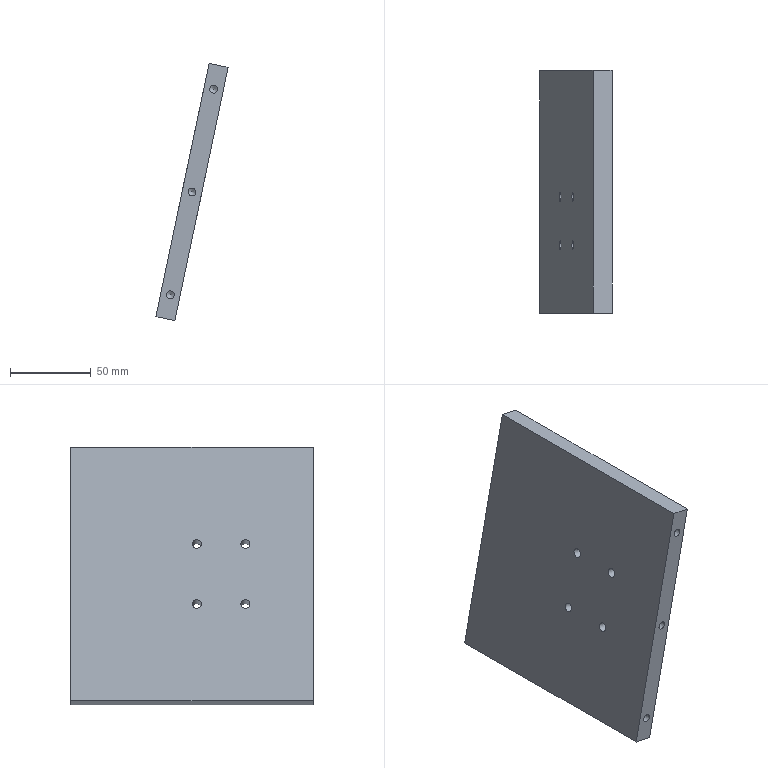Part | STEP file | SN10_007_001-02_PLACA | 1 solid | 22 faces | box 44.646 x 150 x 159.048 mm | volume 285095 mm3 | cylinder 10 | cone 6 | plane 6 | commonest cylinder face diameters 4.917 x6 5.5 x4